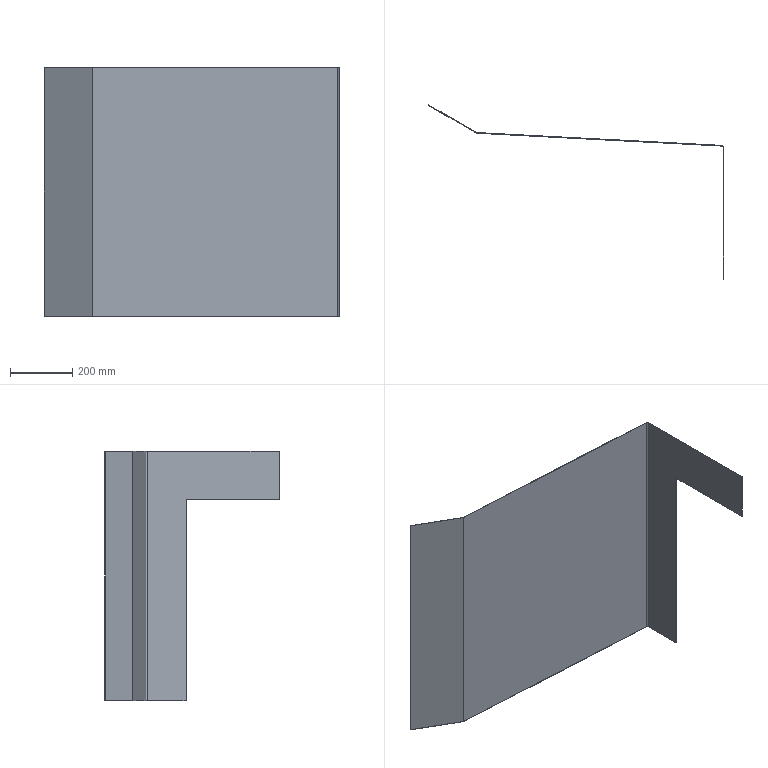Part | SolidWorks | features BaseBody 1 | 1 solid | 30 faces | box 951 x 561.757 x 805 mm | volume 935196 mm3 | plane 22 | cylinder 8 | commonest cylinder face diameters 10 x3 1.473 x2 3.473 x2 12 x1
STEP:
#1=CARTESIAN_POINT('',(478.5,-5.,402.5));
#2=VERTEX_POINT('',#1);
#3=CARTESIAN_POINT('',(477.5,-5.,402.5));
#4=VERTEX_POINT('',#3);
#5=CARTESIAN_POINT('',(478.5,-5.,402.5));
#6=DIRECTION('',(-1.,0.,0.));
#7=VECTOR('',#6,1000.);
#8=LINE('',#5,#7);
#9=EDGE_CURVE('',#2,#4,#8,.T.);
#10=ORIENTED_EDGE('',*,*,#9,.F.);
#11=CARTESIAN_POINT('',(472.544,0.9998,402.5));
#12=VERTEX_POINT('',#11);
#13=CARTESIAN_POINT('',(472.5,-5.,402.5));
#14=DIRECTION('',(0.,0.,1.));
#15=DIRECTION('',(1.,0.,0.));
#16=AXIS2_PLACEMENT_3D('',#13,#14,#15);
#17=CIRCLE('',#16,6.);
#18=EDGE_CURVE('',#2,#12,#17,.T.);
#19=ORIENTED_EDGE('',*,*,#18,.T.);
#20=CARTESIAN_POINT('',(472.536,-0.0001315,402.5));
#21=VERTEX_POINT('',#20);
#22=CARTESIAN_POINT('',(472.544,0.9998,402.5));
#23=DIRECTION('',(-0.007252,-1.,0.));
#24=VECTOR('',#23,1000.);
#25=LINE('',#22,#24);
#26=EDGE_CURVE('',#12,#21,#25,.T.);
#27=ORIENTED_EDGE('',*,*,#26,.T.);
#28=CARTESIAN_POINT('',(472.5,-5.,402.5));
#29=DIRECTION('',(0.,0.,1.));
#30=DIRECTION('',(-1.,0.,0.));
#31=AXIS2_PLACEMENT_3D('',#28,#29,#30);
#32=CIRCLE('',#31,5.);
#33=EDGE_CURVE('',#4,#21,#32,.T.);
#34=ORIENTED_EDGE('',*,*,#33,.F.);
#35=EDGE_LOOP('',(#10,#19,#27,#34));
#36=FACE_OUTER_BOUND('',#35,.T.);
#37=CARTESIAN_POINT('',(478.5,-5.,402.5));
#38=DIRECTION('',(0.,0.,1.));
#39=DIRECTION('',(1.,0.,0.));
#40=AXIS2_PLACEMENT_3D('',#37,#38,#39);
#41=PLANE('',#40);
#42=ADVANCED_FACE('',(#36),#41,.T.);
#43=CARTESIAN_POINT('',(477.5,-5.,-402.5));
#44=VERTEX_POINT('',#43);
#45=CARTESIAN_POINT('',(478.5,-5.,-402.5));
#46=VERTEX_POINT('',#45);
#47=CARTESIAN_POINT('',(477.5,-5.,-402.5));
#48=DIRECTION('',(1.,0.,0.));
#49=VECTOR('',#48,1000.);
#50=LINE('',#47,#49);
#51=EDGE_CURVE('',#44,#46,#50,.T.);
#52=ORIENTED_EDGE('',*,*,#51,.F.);
#53=CARTESIAN_POINT('',(472.536,-0.0001315,-402.5));
#54=VERTEX_POINT('',#53);
#55=CARTESIAN_POINT('',(472.5,-5.,-402.5));
#56=DIRECTION('',(0.,0.,1.));
#57=DIRECTION('',(-1.,0.,0.));
#58=AXIS2_PLACEMENT_3D('',#55,#56,#57);
#59=CIRCLE('',#58,5.);
#60=EDGE_CURVE('',#44,#54,#59,.T.);
#61=ORIENTED_EDGE('',*,*,#60,.T.);
#62=CARTESIAN_POINT('',(472.544,0.9998,-402.5));
#63=VERTEX_POINT('',#62);
#64=CARTESIAN_POINT('',(472.536,-0.0001315,-402.5));
#65=DIRECTION('',(0.007252,1.,0.));
#66=VECTOR('',#65,1000.);
#67=LINE('',#64,#66);
#68=EDGE_CURVE('',#54,#63,#67,.T.);
#69=ORIENTED_EDGE('',*,*,#68,.T.);
#70=CARTESIAN_POINT('',(472.5,-5.,-402.5));
#71=DIRECTION('',(0.,0.,1.));
#72=DIRECTION('',(1.,0.,0.));
#73=AXIS2_PLACEMENT_3D('',#70,#71,#72);
#74=CIRCLE('',#73,6.);
#75=EDGE_CURVE('',#46,#63,#74,.T.);
#76=ORIENTED_EDGE('',*,*,#75,.F.);
#77=EDGE_LOOP('',(#52,#61,#69,#76));
#78=FACE_OUTER_BOUND('',#77,.T.);
#79=CARTESIAN_POINT('',(477.5,-5.,-402.5));
#80=DIRECTION('',(0.,0.,-1.));
#81=DIRECTION('',(-1.,0.,0.));
#82=AXIS2_PLACEMENT_3D('',#79,#80,#81);
#83=PLANE('',#82);
#84=ADVANCED_FACE('',(#78),#83,.T.);
#85=CARTESIAN_POINT('',(472.458,0.002203,402.5));
#86=VERTEX_POINT('',#85);
#87=CARTESIAN_POINT('',(472.51,1.001,402.5));
#88=VERTEX_POINT('',#87);
#89=CARTESIAN_POINT('',(472.458,0.002203,402.5));
#90=DIRECTION('',(0.05234,0.9986,0.));
#91=VECTOR('',#90,1000.);
#92=LINE('',#89,#91);
#93=EDGE_CURVE('',#86,#88,#92,.T.);
#94=ORIENTED_EDGE('',*,*,#93,.F.);
#95=CARTESIAN_POINT('',(472.549,1.736,402.5));
#96=DIRECTION('',(0.,0.,-1.));
#97=DIRECTION('',(1.,0.,0.));
#98=AXIS2_PLACEMENT_3D('',#95,#96,#97);
#99=CIRCLE('',#98,1.737);
#100=EDGE_CURVE('',#21,#86,#99,.T.);
#101=ORIENTED_EDGE('',*,*,#100,.F.);
#102=ORIENTED_EDGE('',*,*,#26,.F.);
#103=CARTESIAN_POINT('',(472.549,1.736,402.5));
#104=DIRECTION('',(0.,0.,-1.));
#105=DIRECTION('',(1.,0.,0.));
#106=AXIS2_PLACEMENT_3D('',#103,#104,#105);
#107=CIRCLE('',#106,0.7366);
#108=EDGE_CURVE('',#12,#88,#107,.T.);
#109=ORIENTED_EDGE('',*,*,#108,.T.);
#110=EDGE_LOOP('',(#94,#101,#102,#109));
#111=FACE_OUTER_BOUND('',#110,.T.);
#112=CARTESIAN_POINT('',(472.458,0.002203,402.5));
#113=DIRECTION('',(0.,0.,1.));
#114=DIRECTION('',(1.,0.,0.));
#115=AXIS2_PLACEMENT_3D('',#112,#113,#114);
#116=PLANE('',#115);
#117=ADVANCED_FACE('',(#111),#116,.T.);
#118=CARTESIAN_POINT('',(-317.084,41.38,402.5));
#119=VERTEX_POINT('',#118);
#120=CARTESIAN_POINT('',(472.5,0.,402.5));
#121=DIRECTION('',(-0.9986,0.05234,0.));
#122=VECTOR('',#121,1000.);
#123=LINE('',#120,#122);
#124=EDGE_CURVE('',#86,#119,#123,.T.);
#125=ORIENTED_EDGE('',*,*,#124,.F.);
#126=ORIENTED_EDGE('',*,*,#93,.T.);
#127=CARTESIAN_POINT('',(-317.031,42.379,402.5));
#128=VERTEX_POINT('',#127);
#129=CARTESIAN_POINT('',(472.552,0.9986,402.5));
#130=DIRECTION('',(-0.9986,0.05234,0.));
#131=VECTOR('',#130,1000.);
#132=LINE('',#129,#131);
#133=EDGE_CURVE('',#88,#128,#132,.T.);
#134=ORIENTED_EDGE('',*,*,#133,.T.);
#135=CARTESIAN_POINT('',(-317.031,42.379,402.5));
#136=DIRECTION('',(-0.05234,-0.9986,0.));
#137=VECTOR('',#136,1000.);
#138=LINE('',#135,#137);
#139=EDGE_CURVE('',#128,#119,#138,.T.);
#140=ORIENTED_EDGE('',*,*,#139,.T.);
#141=EDGE_LOOP('',(#125,#126,#134,#140));
#142=FACE_OUTER_BOUND('',#141,.T.);
#143=CARTESIAN_POINT('',(472.544,0.9998,402.5));
#144=DIRECTION('',(0.,0.,1.));
#145=DIRECTION('',(1.,0.,0.));
#146=AXIS2_PLACEMENT_3D('',#143,#144,#145);
#147=PLANE('',#146);
#148=ADVANCED_FACE('',(#142),#147,.T.);
#149=ORIENTED_EDGE('',*,*,#68,.F.);
#150=CARTESIAN_POINT('',(472.458,0.002203,-402.5));
#151=VERTEX_POINT('',#150);
#152=CARTESIAN_POINT('',(472.549,1.736,-402.5));
#153=DIRECTION('',(0.,0.,-1.));
#154=DIRECTION('',(1.,0.,0.));
#155=AXIS2_PLACEMENT_3D('',#152,#153,#154);
#156=CIRCLE('',#155,1.737);
#157=EDGE_CURVE('',#54,#151,#156,.T.);
#158=ORIENTED_EDGE('',*,*,#157,.T.);
#159=CARTESIAN_POINT('',(472.51,1.001,-402.5));
#160=VERTEX_POINT('',#159);
#161=CARTESIAN_POINT('',(472.51,1.001,-402.5));
#162=DIRECTION('',(-0.05234,-0.9986,0.));
#163=VECTOR('',#162,1000.);
#164=LINE('',#161,#163);
#165=EDGE_CURVE('',#160,#151,#164,.T.);
#166=ORIENTED_EDGE('',*,*,#165,.F.);
#167=CARTESIAN_POINT('',(472.549,1.736,-402.5));
#168=DIRECTION('',(0.,0.,-1.));
#169=DIRECTION('',(1.,0.,0.));
#170=AXIS2_PLACEMENT_3D('',#167,#168,#169);
#171=CIRCLE('',#170,0.7366);
#172=EDGE_CURVE('',#63,#160,#171,.T.);
#173=ORIENTED_EDGE('',*,*,#172,.F.);
#174=EDGE_LOOP('',(#149,#158,#166,#173));
#175=FACE_OUTER_BOUND('',#174,.T.);
#176=CARTESIAN_POINT('',(472.536,-0.0001315,-402.5));
#177=DIRECTION('',(0.,0.,-1.));
#178=DIRECTION('',(-1.,0.,0.));
#179=AXIS2_PLACEMENT_3D('',#176,#177,#178);
#180=PLANE('',#179);
#181=ADVANCED_FACE('',(#175),#180,.T.);
#182=CARTESIAN_POINT('',(477.5,-130.,-402.5));
#183=VERTEX_POINT('',#182);
#184=CARTESIAN_POINT('',(478.5,-130.,-402.5));
#185=VERTEX_POINT('',#184);
#186=CARTESIAN_POINT('',(-237.029,-130.,-402.5));
#187=DIRECTION('',(1.,0.,0.));
#188=VECTOR('',#187,1000.);
#189=LINE('',#186,#188);
#190=EDGE_CURVE('',#183,#185,#189,.T.);
#191=ORIENTED_EDGE('',*,*,#190,.F.);
#192=CARTESIAN_POINT('',(477.5,-5.,-402.5));
#193=DIRECTION('',(0.,1.,0.));
#194=VECTOR('',#193,1000.);
#195=LINE('',#192,#194);
#196=EDGE_CURVE('',#183,#44,#195,.T.);
#197=ORIENTED_EDGE('',*,*,#196,.T.);
#198=ORIENTED_EDGE('',*,*,#51,.T.);
#199=CARTESIAN_POINT('',(478.5,-5.,-402.5));
#200=DIRECTION('',(0.,1.,0.));
#201=VECTOR('',#200,1000.);
#202=LINE('',#199,#201);
#203=EDGE_CURVE('',#185,#46,#202,.T.);
#204=ORIENTED_EDGE('',*,*,#203,.F.);
#205=EDGE_LOOP('',(#191,#197,#198,#204));
#206=FACE_OUTER_BOUND('',#205,.T.);
#207=CARTESIAN_POINT('',(472.51,1.001,-402.5));
#208=DIRECTION('',(0.,0.,-1.));
#209=DIRECTION('',(-1.,0.,0.));
#210=AXIS2_PLACEMENT_3D('',#207,#208,#209);
#211=PLANE('',#210);
#212=ADVANCED_FACE('',(#206),#211,.T.);
#213=CARTESIAN_POINT('',(-317.861,41.611,402.5));
#214=VERTEX_POINT('',#213);
#215=CARTESIAN_POINT('',(-317.361,42.477,402.5));
#216=VERTEX_POINT('',#215);
#217=CARTESIAN_POINT('',(-317.861,41.611,402.5));
#218=DIRECTION('',(0.5,0.866,0.));
#219=VECTOR('',#218,1000.);
#220=LINE('',#217,#219);
#221=EDGE_CURVE('',#214,#216,#220,.T.);
#222=ORIENTED_EDGE('',*,*,#221,.F.);
#223=CARTESIAN_POINT('',(-316.993,43.115,402.5));
#224=DIRECTION('',(0.,0.,-1.));
#225=DIRECTION('',(1.,0.,0.));
#226=AXIS2_PLACEMENT_3D('',#223,#224,#225);
#227=CIRCLE('',#226,1.737);
#228=EDGE_CURVE('',#119,#214,#227,.T.);
#229=ORIENTED_EDGE('',*,*,#228,.F.);
#230=ORIENTED_EDGE('',*,*,#139,.F.);
#231=CARTESIAN_POINT('',(-316.993,43.115,402.5));
#232=DIRECTION('',(0.,0.,-1.));
#233=DIRECTION('',(1.,0.,0.));
#234=AXIS2_PLACEMENT_3D('',#231,#232,#233);
#235=CIRCLE('',#234,0.7366);
#236=EDGE_CURVE('',#128,#216,#235,.T.);
#237=ORIENTED_EDGE('',*,*,#236,.T.);
#238=EDGE_LOOP('',(#222,#229,#230,#237));
#239=FACE_OUTER_BOUND('',#238,.T.);
#240=CARTESIAN_POINT('',(-317.861,41.611,402.5));
#241=DIRECTION('',(0.,0.,1.));
#242=DIRECTION('',(1.,0.,0.));
#243=AXIS2_PLACEMENT_3D('',#240,#241,#242);
#244=PLANE('',#243);
#245=ADVANCED_FACE('',(#239),#244,.T.);
#246=CARTESIAN_POINT('',(-467.67,129.257,402.5));
#247=VERTEX_POINT('',#246);
#248=CARTESIAN_POINT('',(-317.,42.268,402.5));
#249=DIRECTION('',(-0.866,0.5,0.));
#250=VECTOR('',#249,1000.);
#251=LINE('',#248,#250);
#252=EDGE_CURVE('',#216,#247,#251,.T.);
#253=ORIENTED_EDGE('',*,*,#252,.T.);
#254=CARTESIAN_POINT('',(-468.17,128.391,402.5));
#255=VERTEX_POINT('',#254);
#256=CARTESIAN_POINT('',(-467.63,129.327,402.5));
#257=DIRECTION('',(-0.5,-0.866,0.));
#258=VECTOR('',#257,1000.);
#259=LINE('',#256,#258);
#260=EDGE_CURVE('',#247,#255,#259,.T.);
#261=ORIENTED_EDGE('',*,*,#260,.T.);
#262=CARTESIAN_POINT('',(-317.5,41.402,402.5));
#263=DIRECTION('',(-0.866,0.5,0.));
#264=VECTOR('',#263,1000.);
#265=LINE('',#262,#264);
#266=EDGE_CURVE('',#214,#255,#265,.T.);
#267=ORIENTED_EDGE('',*,*,#266,.F.);
#268=ORIENTED_EDGE('',*,*,#221,.T.);
#269=EDGE_LOOP('',(#253,#261,#267,#268));
#270=FACE_OUTER_BOUND('',#269,.T.);
#271=CARTESIAN_POINT('',(-317.031,42.379,402.5));
#272=DIRECTION('',(0.,0.,1.));
#273=DIRECTION('',(1.,0.,0.));
#274=AXIS2_PLACEMENT_3D('',#271,#272,#273);
#275=PLANE('',#274);
#276=ADVANCED_FACE('',(#270),#275,.T.);
#277=CARTESIAN_POINT('',(-317.084,41.38,-402.5));
#278=VERTEX_POINT('',#277);
#279=CARTESIAN_POINT('',(-317.031,42.379,-402.5));
#280=VERTEX_POINT('',#279);
#281=CARTESIAN_POINT('',(-317.084,41.38,-402.5));
#282=DIRECTION('',(0.05234,0.9986,0.));
#283=VECTOR('',#282,1000.);
#284=LINE('',#281,#283);
#285=EDGE_CURVE('',#278,#280,#284,.T.);
#286=ORIENTED_EDGE('',*,*,#285,.F.);
#287=CARTESIAN_POINT('',(-317.861,41.611,-402.5));
#288=VERTEX_POINT('',#287);
#289=CARTESIAN_POINT('',(-316.993,43.115,-402.5));
#290=DIRECTION('',(0.,0.,-1.));
#291=DIRECTION('',(1.,0.,0.));
#292=AXIS2_PLACEMENT_3D('',#289,#290,#291);
#293=CIRCLE('',#292,1.737);
#294=EDGE_CURVE('',#278,#288,#293,.T.);
#295=ORIENTED_EDGE('',*,*,#294,.T.);
#296=CARTESIAN_POINT('',(-317.361,42.477,-402.5));
#297=VERTEX_POINT('',#296);
#298=CARTESIAN_POINT('',(-317.361,42.477,-402.5));
#299=DIRECTION('',(-0.5,-0.866,0.));
#300=VECTOR('',#299,1000.);
#301=LINE('',#298,#300);
#302=EDGE_CURVE('',#297,#288,#301,.T.);
#303=ORIENTED_EDGE('',*,*,#302,.F.);
#304=CARTESIAN_POINT('',(-316.993,43.115,-402.5));
#305=DIRECTION('',(0.,0.,-1.));
#306=DIRECTION('',(1.,0.,0.));
#307=AXIS2_PLACEMENT_3D('',#304,#305,#306);
#308=CIRCLE('',#307,0.7366);
#309=EDGE_CURVE('',#280,#297,#308,.T.);
#310=ORIENTED_EDGE('',*,*,#309,.F.);
#311=EDGE_LOOP('',(#286,#295,#303,#310));
#312=FACE_OUTER_BOUND('',#311,.T.);
#313=CARTESIAN_POINT('',(-317.084,41.38,-402.5));
#314=DIRECTION('',(0.,0.,-1.));
#315=DIRECTION('',(-1.,0.,0.));
#316=AXIS2_PLACEMENT_3D('',#313,#314,#315);
#317=PLANE('',#316);
#318=ADVANCED_FACE('',(#312),#317,.T.);
#319=CARTESIAN_POINT('',(472.5,0.,-402.5));
#320=DIRECTION('',(-0.9986,0.05234,0.));
#321=VECTOR('',#320,1000.);
#322=LINE('',#319,#321);
#323=EDGE_CURVE('',#151,#278,#322,.T.);
#324=ORIENTED_EDGE('',*,*,#323,.T.);
#325=ORIENTED_EDGE('',*,*,#285,.T.);
#326=CARTESIAN_POINT('',(472.552,0.9986,-402.5));
#327=DIRECTION('',(-0.9986,0.05234,0.));
#328=VECTOR('',#327,1000.);
#329=LINE('',#326,#328);
#330=EDGE_CURVE('',#160,#280,#329,.T.);
#331=ORIENTED_EDGE('',*,*,#330,.F.);
#332=ORIENTED_EDGE('',*,*,#165,.T.);
#333=EDGE_LOOP('',(#324,#325,#331,#332));
#334=FACE_OUTER_BOUND('',#333,.T.);
#335=CARTESIAN_POINT('',(-317.361,42.477,-402.5));
#336=DIRECTION('',(0.,0.,-1.));
#337=DIRECTION('',(-1.,0.,0.));
#338=AXIS2_PLACEMENT_3D('',#335,#336,#337);
#339=PLANE('',#338);
#340=ADVANCED_FACE('',(#334),#339,.T.);
#341=CARTESIAN_POINT('',(-467.67,129.257,-402.5));
#342=VERTEX_POINT('',#341);
#343=CARTESIAN_POINT('',(-317.,42.268,-402.5));
#344=DIRECTION('',(-0.866,0.5,0.));
#345=VECTOR('',#344,1000.);
#346=LINE('',#343,#345);
#347=EDGE_CURVE('',#297,#342,#346,.T.);
#348=ORIENTED_EDGE('',*,*,#347,.T.);
#349=CARTESIAN_POINT('',(-472.,131.757,-397.5));
#350=VERTEX_POINT('',#349);
#351=CARTESIAN_POINT('',(-467.67,129.257,-397.5));
#352=DIRECTION('',(0.5,0.866,0.));
#353=DIRECTION('',(0.866,-0.5,0.));
#354=AXIS2_PLACEMENT_3D('',#351,#352,#353);
#355=CIRCLE('',#354,5.);
#356=EDGE_CURVE('',#342,#350,#355,.T.);
#357=ORIENTED_EDGE('',*,*,#356,.T.);
#358=CARTESIAN_POINT('',(-472.,131.757,397.5));
#359=VERTEX_POINT('',#358);
#360=CARTESIAN_POINT('',(-472.,131.757,402.5));
#361=DIRECTION('',(0.,0.,-1.));
#362=VECTOR('',#361,1000.);
#363=LINE('',#360,#362);
#364=EDGE_CURVE('',#359,#350,#363,.T.);
#365=ORIENTED_EDGE('',*,*,#364,.F.);
#366=CARTESIAN_POINT('',(-467.67,129.257,397.5));
#367=DIRECTION('',(0.5,0.866,0.));
#368=DIRECTION('',(0.866,-0.5,0.));
#369=AXIS2_PLACEMENT_3D('',#366,#367,#368);
#370=CIRCLE('',#369,5.);
#371=EDGE_CURVE('',#359,#247,#370,.T.);
#372=ORIENTED_EDGE('',*,*,#371,.T.);
#373=ORIENTED_EDGE('',*,*,#252,.F.);
#374=CARTESIAN_POINT('',(-317.361,42.477,402.5));
#375=DIRECTION('',(0.,0.,-1.));
#376=VECTOR('',#375,1000.);
#377=LINE('',#374,#376);
#378=EDGE_CURVE('',#216,#297,#377,.T.);
#379=ORIENTED_EDGE('',*,*,#378,.T.);
#380=EDGE_LOOP('',(#348,#357,#365,#372,#373,#379));
#381=FACE_OUTER_BOUND('',#380,.T.);
#382=CARTESIAN_POINT('',(-317.,42.268,402.5));
#383=DIRECTION('',(-0.5,-0.866,0.));
#384=DIRECTION('',(0.866,-0.5,0.));
#385=AXIS2_PLACEMENT_3D('',#382,#383,#384);
#386=PLANE('',#385);
#387=ADVANCED_FACE('',(#381),#386,.F.);
#388=ORIENTED_EDGE('',*,*,#364,.T.);
#389=CARTESIAN_POINT('',(-472.5,130.891,-397.5));
#390=VERTEX_POINT('',#389);
#391=CARTESIAN_POINT('',(-472.5,130.891,-397.5));
#392=DIRECTION('',(-0.5,-0.866,0.));
#393=VECTOR('',#392,1000.);
#394=LINE('',#391,#393);
#395=EDGE_CURVE('',#350,#390,#394,.T.);
#396=ORIENTED_EDGE('',*,*,#395,.T.);
#397=CARTESIAN_POINT('',(-472.5,130.891,397.5));
#398=VERTEX_POINT('',#397);
#399=CARTESIAN_POINT('',(-472.5,130.891,402.5));
#400=DIRECTION('',(0.,0.,-1.));
#401=VECTOR('',#400,1000.);
#402=LINE('',#399,#401);
#403=EDGE_CURVE('',#398,#390,#402,.T.);
#404=ORIENTED_EDGE('',*,*,#403,.F.);
#405=CARTESIAN_POINT('',(-472.5,130.891,397.5));
#406=DIRECTION('',(0.5,0.866,0.));
#407=VECTOR('',#406,1000.);
#408=LINE('',#405,#407);
#409=EDGE_CURVE('',#398,#359,#408,.T.);
#410=ORIENTED_EDGE('',*,*,#409,.T.);
#411=EDGE_LOOP('',(#388,#396,#404,#410));
#412=FACE_OUTER_BOUND('',#411,.T.);
#413=CARTESIAN_POINT('',(-472.5,130.891,402.5));
#414=DIRECTION('',(-0.866,0.5,0.));
#415=DIRECTION('',(-0.5,-0.866,0.));
#416=AXIS2_PLACEMENT_3D('',#413,#414,#415);
#417=PLANE('',#416);
#418=ADVANCED_FACE('',(#412),#417,.T.);
#419=ORIENTED_EDGE('',*,*,#403,.T.);
#420=CARTESIAN_POINT('',(-468.17,128.391,-402.5));
#421=VERTEX_POINT('',#420);
#422=CARTESIAN_POINT('',(-468.17,128.391,-397.5));
#423=DIRECTION('',(-0.5,-0.866,0.));
#424=DIRECTION('',(0.866,-0.5,0.));
#425=AXIS2_PLACEMENT_3D('',#422,#423,#424);
#426=CIRCLE('',#425,5.);
#427=EDGE_CURVE('',#390,#421,#426,.T.);
#428=ORIENTED_EDGE('',*,*,#427,.T.);
#429=CARTESIAN_POINT('',(-317.5,41.402,-402.5));
#430=DIRECTION('',(-0.866,0.5,0.));
#431=VECTOR('',#430,1000.);
#432=LINE('',#429,#431);
#433=EDGE_CURVE('',#288,#421,#432,.T.);
#434=ORIENTED_EDGE('',*,*,#433,.F.);
#435=CARTESIAN_POINT('',(-317.861,41.611,402.5));
#436=DIRECTION('',(0.,0.,-1.));
#437=VECTOR('',#436,1000.);
#438=LINE('',#435,#437);
#439=EDGE_CURVE('',#214,#288,#438,.T.);
#440=ORIENTED_EDGE('',*,*,#439,.F.);
#441=ORIENTED_EDGE('',*,*,#266,.T.);
#442=CARTESIAN_POINT('',(-468.17,128.391,397.5));
#443=DIRECTION('',(-0.5,-0.866,0.));
#444=DIRECTION('',(0.866,-0.5,0.));
#445=AXIS2_PLACEMENT_3D('',#442,#443,#444);
#446=CIRCLE('',#445,5.);
#447=EDGE_CURVE('',#255,#398,#446,.T.);
#448=ORIENTED_EDGE('',*,*,#447,.T.);
#449=EDGE_LOOP('',(#419,#428,#434,#440,#441,#448));
#450=FACE_OUTER_BOUND('',#449,.T.);
#451=CARTESIAN_POINT('',(-317.5,41.402,402.5));
#452=DIRECTION('',(-0.5,-0.866,0.));
#453=DIRECTION('',(0.866,-0.5,0.));
#454=AXIS2_PLACEMENT_3D('',#451,#452,#453);
#455=PLANE('',#454);
#456=ADVANCED_FACE('',(#450),#455,.T.);
#457=ORIENTED_EDGE('',*,*,#294,.F.);
#458=CARTESIAN_POINT('',(-317.084,41.38,402.5));
#459=DIRECTION('',(0.,0.,-1.));
#460=VECTOR('',#459,1000.);
#461=LINE('',#458,#460);
#462=EDGE_CURVE('',#119,#278,#461,.T.);
#463=ORIENTED_EDGE('',*,*,#462,.F.);
#464=ORIENTED_EDGE('',*,*,#228,.T.);
#465=ORIENTED_EDGE('',*,*,#439,.T.);
#466=EDGE_LOOP('',(#457,#463,#464,#465));
#467=FACE_OUTER_BOUND('',#466,.T.);
#468=CARTESIAN_POINT('',(-316.993,43.115,402.5));
#469=DIRECTION('',(0.,0.,-1.));
#470=DIRECTION('',(-1.,0.,0.));
#471=AXIS2_PLACEMENT_3D('',#468,#469,#470);
#472=CYLINDRICAL_SURFACE('',#471,1.737);
#473=ADVANCED_FACE('',(#467),#472,.T.);
#474=ORIENTED_EDGE('',*,*,#323,.F.);
#475=CARTESIAN_POINT('',(472.458,0.002203,402.5));
#476=DIRECTION('',(0.,0.,-1.));
#477=VECTOR('',#476,1000.);
#478=LINE('',#475,#477);
#479=EDGE_CURVE('',#86,#151,#478,.T.);
#480=ORIENTED_EDGE('',*,*,#479,.F.);
#481=ORIENTED_EDGE('',*,*,#124,.T.);
#482=ORIENTED_EDGE('',*,*,#462,.T.);
#483=EDGE_LOOP('',(#474,#480,#481,#482));
#484=FACE_OUTER_BOUND('',#483,.T.);
#485=CARTESIAN_POINT('',(472.5,0.,402.5));
#486=DIRECTION('',(-0.05234,-0.9986,0.));
#487=DIRECTION('',(0.9986,-0.05234,0.));
#488=AXIS2_PLACEMENT_3D('',#485,#486,#487);
#489=PLANE('',#488);
#490=ADVANCED_FACE('',(#484),#489,.T.);
#491=ORIENTED_EDGE('',*,*,#157,.F.);
#492=CARTESIAN_POINT('',(472.536,-0.0001315,402.5));
#493=DIRECTION('',(0.,0.,-1.));
#494=VECTOR('',#493,1000.);
#495=LINE('',#492,#494);
#496=EDGE_CURVE('',#21,#54,#495,.T.);
#497=ORIENTED_EDGE('',*,*,#496,.F.);
#498=ORIENTED_EDGE('',*,*,#100,.T.);
#499=ORIENTED_EDGE('',*,*,#479,.T.);
#500=EDGE_LOOP('',(#491,#497,#498,#499));
#501=FACE_OUTER_BOUND('',#500,.T.);
#502=CARTESIAN_POINT('',(472.549,1.736,402.5));
#503=DIRECTION('',(0.,0.,-1.));
#504=DIRECTION('',(-1.,0.,0.));
#505=AXIS2_PLACEMENT_3D('',#502,#503,#504);
#506=CYLINDRICAL_SURFACE('',#505,1.737);
#507=ADVANCED_FACE('',(#501),#506,.T.);
#508=ORIENTED_EDGE('',*,*,#60,.F.);
#509=CARTESIAN_POINT('',(477.5,-5.,402.5));
#510=DIRECTION('',(0.,0.,-1.));
#511=VECTOR('',#510,1000.);
#512=LINE('',#509,#511);
#513=EDGE_CURVE('',#4,#44,#512,.T.);
#514=ORIENTED_EDGE('',*,*,#513,.F.);
#515=ORIENTED_EDGE('',*,*,#33,.T.);
#516=ORIENTED_EDGE('',*,*,#496,.T.);
#517=EDGE_LOOP('',(#508,#514,#515,#516));
#518=FACE_OUTER_BOUND('',#517,.T.);
#519=CARTESIAN_POINT('',(472.5,-5.,402.5));
#520=DIRECTION('',(0.,0.,-1.));
#521=DIRECTION('',(-1.,0.,0.));
#522=AXIS2_PLACEMENT_3D('',#519,#520,#521);
#523=CYLINDRICAL_SURFACE('',#522,5.);
#524=ADVANCED_FACE('',(#518),#523,.F.);
#525=CARTESIAN_POINT('',(477.5,-130.,246.));
#526=VERTEX_POINT('',#525);
#527=CARTESIAN_POINT('',(477.5,-130.,246.));
#528=DIRECTION('',(0.,0.,1.));
#529=VECTOR('',#528,1000.);
#530=LINE('',#527,#529);
#531=EDGE_CURVE('',#183,#526,#530,.T.);
#532=ORIENTED_EDGE('',*,*,#531,.T.);
#533=CARTESIAN_POINT('',(477.5,-430.,246.));
#534=VERTEX_POINT('',#533);
#535=CARTESIAN_POINT('',(477.5,-130.,246.));
#536=DIRECTION('',(0.,-1.,0.));
#537=VECTOR('',#536,1000.);
#538=LINE('',#535,#537);
#539=EDGE_CURVE('',#526,#534,#538,.T.);
#540=ORIENTED_EDGE('',*,*,#539,.T.);
#541=CARTESIAN_POINT('',(477.5,-430.,402.5));
#542=VERTEX_POINT('',#541);
#543=CARTESIAN_POINT('',(477.5,-430.,402.5));
#544=DIRECTION('',(0.,0.,-1.));
#545=VECTOR('',#544,1000.);
#546=LINE('',#543,#545);
#547=EDGE_CURVE('',#542,#534,#546,.T.);
#548=ORIENTED_EDGE('',*,*,#547,.F.);
#549=CARTESIAN_POINT('',(477.5,-5.,402.5));
#550=DIRECTION('',(0.,1.,0.));
#551=VECTOR('',#550,1000.);
#552=LINE('',#549,#551);
#553=EDGE_CURVE('',#542,#4,#552,.T.);
#554=ORIENTED_EDGE('',*,*,#553,.T.);
#555=ORIENTED_EDGE('',*,*,#513,.T.);
#556=ORIENTED_EDGE('',*,*,#196,.F.);
#557=EDGE_LOOP('',(#532,#540,#548,#554,#555,#556));
#558=FACE_OUTER_BOUND('',#557,.T.);
#559=CARTESIAN_POINT('',(477.5,-5.,402.5));
#560=DIRECTION('',(-1.,0.,0.));
#561=DIRECTION('',(0.,-1.,0.));
#562=AXIS2_PLACEMENT_3D('',#559,#560,#561);
#563=PLANE('',#562);
#564=ADVANCED_FACE('',(#558),#563,.T.);
#565=CARTESIAN_POINT('',(478.5,-430.,246.));
#566=VERTEX_POINT('',#565);
#567=CARTESIAN_POINT('',(-237.029,-430.,246.));
#568=DIRECTION('',(1.,0.,0.));
#569=VECTOR('',#568,1000.);
#570=LINE('',#567,#569);
#571=EDGE_CURVE('',#534,#566,#570,.T.);
#572=ORIENTED_EDGE('',*,*,#571,.T.);
#573=CARTESIAN_POINT('',(478.5,-430.,402.5));
#574=VERTEX_POINT('',#573);
#575=CARTESIAN_POINT('',(478.5,-430.,402.5));
#576=DIRECTION('',(0.,0.,-1.));
#577=VECTOR('',#576,1000.);
#578=LINE('',#575,#577);
#579=EDGE_CURVE('',#574,#566,#578,.T.);
#580=ORIENTED_EDGE('',*,*,#579,.F.);
#581=CARTESIAN_POINT('',(478.5,-430.,402.5));
#582=DIRECTION('',(-1.,0.,0.));
#583=VECTOR('',#582,1000.);
#584=LINE('',#581,#583);
#585=EDGE_CURVE('',#574,#542,#584,.T.);
#586=ORIENTED_EDGE('',*,*,#585,.T.);
#587=ORIENTED_EDGE('',*,*,#547,.T.);
#588=EDGE_LOOP('',(#572,#580,#586,#587));
#589=FACE_OUTER_BOUND('',#588,.T.);
#590=CARTESIAN_POINT('',(478.5,-430.,402.5));
#591=DIRECTION('',(0.,-1.,0.));
#592=DIRECTION('',(0.,0.,-1.));
#593=AXIS2_PLACEMENT_3D('',#590,#591,#592);
#594=PLANE('',#593);
#595=ADVANCED_FACE('',(#589),#594,.T.);
#596=CARTESIAN_POINT('',(478.5,-130.,246.));
#597=VERTEX_POINT('',#596);
#598=CARTESIAN_POINT('',(478.5,-130.,246.));
#599=DIRECTION('',(0.,-1.,0.));
#600=VECTOR('',#599,1000.);
#601=LINE('',#598,#600);
#602=EDGE_CURVE('',#597,#566,#601,.T.);
#603=ORIENTED_EDGE('',*,*,#602,.F.);
#604=CARTESIAN_POINT('',(478.5,-130.,246.));
#605=DIRECTION('',(0.,0.,1.));
#606=VECTOR('',#605,1000.);
#607=LINE('',#604,#606);
#608=EDGE_CURVE('',#185,#597,#607,.T.);
#609=ORIENTED_EDGE('',*,*,#608,.F.);
#610=ORIENTED_EDGE('',*,*,#203,.T.);
#611=CARTESIAN_POINT('',(478.5,-5.,402.5));
#612=DIRECTION('',(0.,0.,-1.));
#613=VECTOR('',#612,1000.);
#614=LINE('',#611,#613);
#615=EDGE_CURVE('',#2,#46,#614,.T.);
#616=ORIENTED_EDGE('',*,*,#615,.F.);
#617=CARTESIAN_POINT('',(478.5,-5.,402.5));
#618=DIRECTION('',(0.,1.,0.));
#619=VECTOR('',#618,1000.);
#620=LINE('',#617,#619);
#621=EDGE_CURVE('',#574,#2,#620,.T.);
#622=ORIENTED_EDGE('',*,*,#621,.F.);
#623=ORIENTED_EDGE('',*,*,#579,.T.);
#624=EDGE_LOOP('',(#603,#609,#610,#616,#622,#623));
#625=FACE_OUTER_BOUND('',#624,.T.);
#626=CARTESIAN_POINT('',(478.5,-5.,402.5));
#627=DIRECTION('',(-1.,0.,0.));
#628=DIRECTION('',(0.,-1.,0.));
#629=AXIS2_PLACEMENT_3D('',#626,#627,#628);
#630=PLANE('',#629);
#631=ADVANCED_FACE('',(#625),#630,.F.);
#632=ORIENTED_EDGE('',*,*,#75,.T.);
#633=CARTESIAN_POINT('',(472.544,0.9998,402.5));
#634=DIRECTION('',(0.,0.,-1.));
#635=VECTOR('',#634,1000.);
#636=LINE('',#633,#635);
#637=EDGE_CURVE('',#12,#63,#636,.T.);
#638=ORIENTED_EDGE('',*,*,#637,.F.);
#639=ORIENTED_EDGE('',*,*,#18,.F.);
#640=ORIENTED_EDGE('',*,*,#615,.T.);
#641=EDGE_LOOP('',(#632,#638,#639,#640));
#642=FACE_OUTER_BOUND('',#641,.T.);
#643=CARTESIAN_POINT('',(472.5,-5.,402.5));
#644=DIRECTION('',(0.,0.,-1.));
#645=DIRECTION('',(-1.,0.,0.));
#646=AXIS2_PLACEMENT_3D('',#643,#644,#645);
#647=CYLINDRICAL_SURFACE('',#646,6.);
#648=ADVANCED_FACE('',(#642),#647,.T.);
#649=ORIENTED_EDGE('',*,*,#172,.T.);
#650=CARTESIAN_POINT('',(472.51,1.001,402.5));
#651=DIRECTION('',(0.,0.,-1.));
#652=VECTOR('',#651,1000.);
#653=LINE('',#650,#652);
#654=EDGE_CURVE('',#88,#160,#653,.T.);
#655=ORIENTED_EDGE('',*,*,#654,.F.);
#656=ORIENTED_EDGE('',*,*,#108,.F.);
#657=ORIENTED_EDGE('',*,*,#637,.T.);
#658=EDGE_LOOP('',(#649,#655,#656,#657));
#659=FACE_OUTER_BOUND('',#658,.T.);
#660=CARTESIAN_POINT('',(472.549,1.736,402.5));
#661=DIRECTION('',(0.,0.,-1.));
#662=DIRECTION('',(-1.,0.,0.));
#663=AXIS2_PLACEMENT_3D('',#660,#661,#662);
#664=CYLINDRICAL_SURFACE('',#663,0.7366);
#665=ADVANCED_FACE('',(#659),#664,.F.);
#666=ORIENTED_EDGE('',*,*,#330,.T.);
#667=CARTESIAN_POINT('',(-317.031,42.379,402.5));
#668=DIRECTION('',(0.,0.,-1.));
#669=VECTOR('',#668,1000.);
#670=LINE('',#667,#669);
#671=EDGE_CURVE('',#128,#280,#670,.T.);
#672=ORIENTED_EDGE('',*,*,#671,.F.);
#673=ORIENTED_EDGE('',*,*,#133,.F.);
#674=ORIENTED_EDGE('',*,*,#654,.T.);
#675=EDGE_LOOP('',(#666,#672,#673,#674));
#676=FACE_OUTER_BOUND('',#675,.T.);
#677=CARTESIAN_POINT('',(472.552,0.9986,402.5));
#678=DIRECTION('',(-0.05234,-0.9986,0.));
#679=DIRECTION('',(0.9986,-0.05234,0.));
#680=AXIS2_PLACEMENT_3D('',#677,#678,#679);
#681=PLANE('',#680);
#682=ADVANCED_FACE('',(#676),#681,.F.);
#683=ORIENTED_EDGE('',*,*,#309,.T.);
#684=ORIENTED_EDGE('',*,*,#378,.F.);
#685=ORIENTED_EDGE('',*,*,#236,.F.);
#686=ORIENTED_EDGE('',*,*,#671,.T.);
#687=EDGE_LOOP('',(#683,#684,#685,#686));
#688=FACE_OUTER_BOUND('',#687,.T.);
#689=CARTESIAN_POINT('',(-316.993,43.115,402.5));
#690=DIRECTION('',(0.,0.,-1.));
#691=DIRECTION('',(-1.,0.,0.));
#692=AXIS2_PLACEMENT_3D('',#689,#690,#691);
#693=CYLINDRICAL_SURFACE('',#692,0.7366);
#694=ADVANCED_FACE('',(#688),#693,.F.);
#695=ORIENTED_EDGE('',*,*,#621,.T.);
#696=ORIENTED_EDGE('',*,*,#9,.T.);
#697=ORIENTED_EDGE('',*,*,#553,.F.);
#698=ORIENTED_EDGE('',*,*,#585,.F.);
#699=EDGE_LOOP('',(#695,#696,#697,#698));
#700=FACE_OUTER_BOUND('',#699,.T.);
#701=CARTESIAN_POINT('',(-316.993,43.115,402.5));
#702=DIRECTION('',(0.,0.,1.));
#703=DIRECTION('',(1.,0.,0.));
#704=AXIS2_PLACEMENT_3D('',#701,#702,#703);
#705=PLANE('',#704);
#706=ADVANCED_FACE('',(#700),#705,.T.);
#707=ORIENTED_EDGE('',*,*,#433,.T.);
#708=CARTESIAN_POINT('',(-467.67,129.257,-402.5));
#709=DIRECTION('',(0.5,0.866,0.));
#710=VECTOR('',#709,1000.);
#711=LINE('',#708,#710);
#712=EDGE_CURVE('',#421,#342,#711,.T.);
#713=ORIENTED_EDGE('',*,*,#712,.T.);
#714=ORIENTED_EDGE('',*,*,#347,.F.);
#715=ORIENTED_EDGE('',*,*,#302,.T.);
#716=EDGE_LOOP('',(#707,#713,#714,#715));
#717=FACE_OUTER_BOUND('',#716,.T.);
#718=CARTESIAN_POINT('',(-316.993,43.115,-402.5));
#719=DIRECTION('',(0.,0.,1.));
#720=DIRECTION('',(1.,0.,0.));
#721=AXIS2_PLACEMENT_3D('',#718,#719,#720);
#722=PLANE('',#721);
#723=ADVANCED_FACE('',(#717),#722,.F.);
#724=ORIENTED_EDGE('',*,*,#427,.F.);
#725=ORIENTED_EDGE('',*,*,#395,.F.);
#726=ORIENTED_EDGE('',*,*,#356,.F.);
#727=ORIENTED_EDGE('',*,*,#712,.F.);
#728=EDGE_LOOP('',(#724,#725,#726,#727));
#729=FACE_OUTER_BOUND('',#728,.T.);
#730=CARTESIAN_POINT('',(-467.302,129.895,-397.5));
#731=DIRECTION('',(-0.5,-0.866,0.));
#732=DIRECTION('',(0.866,-0.5,0.));
#733=AXIS2_PLACEMENT_3D('',#730,#731,#732);
#734=CYLINDRICAL_SURFACE('',#733,5.);
#735=ADVANCED_FACE('',(#729),#734,.T.);
#736=ORIENTED_EDGE('',*,*,#447,.F.);
#737=ORIENTED_EDGE('',*,*,#260,.F.);
#738=ORIENTED_EDGE('',*,*,#371,.F.);
#739=ORIENTED_EDGE('',*,*,#409,.F.);
#740=EDGE_LOOP('',(#736,#737,#738,#739));
#741=FACE_OUTER_BOUND('',#740,.T.);
#742=CARTESIAN_POINT('',(-468.17,128.391,397.5));
#743=DIRECTION('',(0.5,0.866,0.));
#744=DIRECTION('',(-0.866,0.5,0.));
#745=AXIS2_PLACEMENT_3D('',#742,#743,#744);
#746=CYLINDRICAL_SURFACE('',#745,5.);
#747=ADVANCED_FACE('',(#741),#746,.T.);
#748=ORIENTED_EDGE('',*,*,#190,.T.);
#749=ORIENTED_EDGE('',*,*,#608,.T.);
#750=CARTESIAN_POINT('',(-237.029,-130.,246.));
#751=DIRECTION('',(1.,0.,0.));
#752=VECTOR('',#751,1000.);
#753=LINE('',#750,#752);
#754=EDGE_CURVE('',#526,#597,#753,.T.);
#755=ORIENTED_EDGE('',*,*,#754,.F.);
#756=ORIENTED_EDGE('',*,*,#531,.F.);
#757=EDGE_LOOP('',(#748,#749,#755,#756));
#758=FACE_OUTER_BOUND('',#757,.T.);
#759=CARTESIAN_POINT('',(-237.029,-130.,246.));
#760=DIRECTION('',(0.,1.,0.));
#761=DIRECTION('',(-1.,0.,0.));
#762=AXIS2_PLACEMENT_3D('',#759,#760,#761);
#763=PLANE('',#762);
#764=ADVANCED_FACE('',(#758),#763,.F.);
#765=ORIENTED_EDGE('',*,*,#754,.T.);
#766=ORIENTED_EDGE('',*,*,#602,.T.);
#767=ORIENTED_EDGE('',*,*,#571,.F.);
#768=ORIENTED_EDGE('',*,*,#539,.F.);
#769=EDGE_LOOP('',(#765,#766,#767,#768));
#770=FACE_OUTER_BOUND('',#769,.T.);
#771=CARTESIAN_POINT('',(-237.029,-130.,246.));
#772=DIRECTION('',(0.,0.,1.));
#773=DIRECTION('',(0.,-1.,0.));
#774=AXIS2_PLACEMENT_3D('',#771,#772,#773);
#775=PLANE('',#774);
#776=ADVANCED_FACE('',(#770),#775,.F.);
#777=CLOSED_SHELL('',(#42,#84,#117,#148,#181,#212,#245,#276,#318,#340,#387,#418,#456,#473,#490,#507,#524,#564,#595,#631,#648,#665,#682,#694,#706,#723,#735,#747,#764,#776));
#778=MANIFOLD_SOLID_BREP('',#777);
#779=CARTESIAN_POINT('',(0.,0.,0.));
#780=DIRECTION('',(0.,0.,1.));
#781=DIRECTION('',(1.,0.,0.));
#782=AXIS2_PLACEMENT_3D('',#779,#780,#781);
#783=(LENGTH_UNIT()NAMED_UNIT(*)SI_UNIT(.MILLI.,.METRE.));
#784=UNCERTAINTY_MEASURE_WITH_UNIT(LENGTH_MEASURE(0.00001),#783,'','');
#785=(NAMED_UNIT(*)PLANE_ANGLE_UNIT()SI_UNIT($,.RADIAN.));
#786=(NAMED_UNIT(*)SI_UNIT($,.STERADIAN.)SOLID_ANGLE_UNIT());
#787=(GEOMETRIC_REPRESENTATION_CONTEXT(3)GLOBAL_UNCERTAINTY_ASSIGNED_CONTEXT((#784))GLOBAL_UNIT_ASSIGNED_CONTEXT((#783,#785,#786))REPRESENTATION_CONTEXT('',''));
#788=ADVANCED_BREP_SHAPE_REPRESENTATION('',(#778,#782),#787);